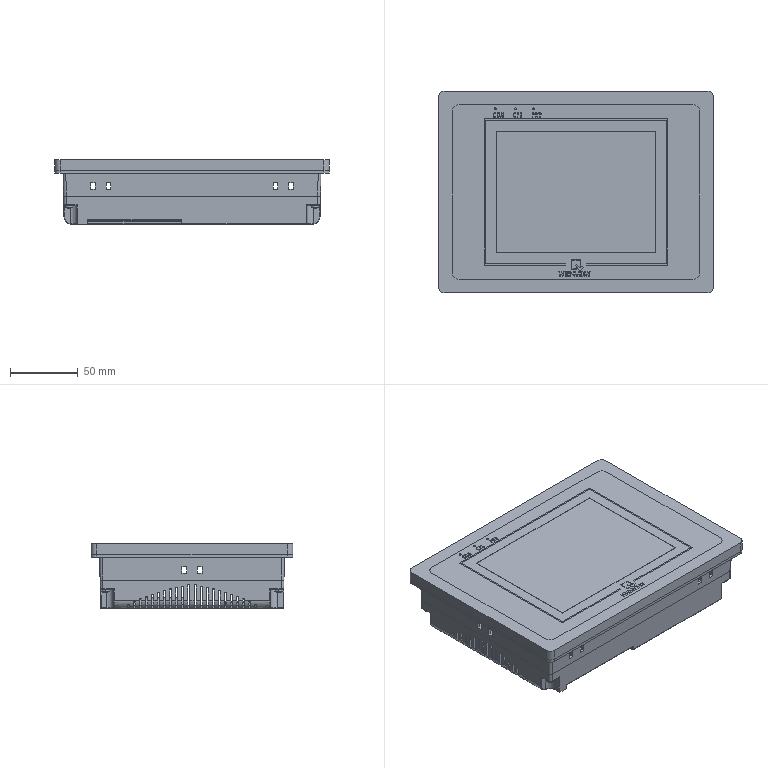Part | SolidWorks | 33 solids | 1384 faces | box 203 x 149 x 48 mm | volume 360474 mm3 | plane 773 | cylinder 437 | spline 130 | torus 20 | sphere 16 | cone 8 | commonest cylinder face diameters 1 x77 3 x52 8 x46 12 x44 2 x36 4 x32